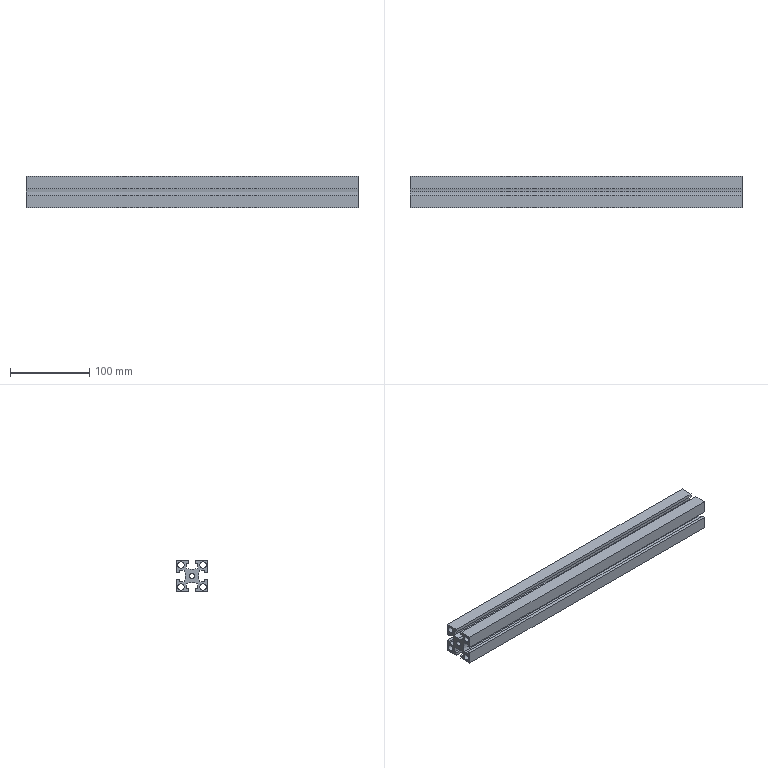Part | STEP file | PN_0063 (cross stop) | 1 solid | 49 faces | box 420 x 40 x 40 mm | volume 346994 mm3 | plane 34 | cylinder 15 | commonest cylinder face diameters 8 x8 30 x5 6.7 x2